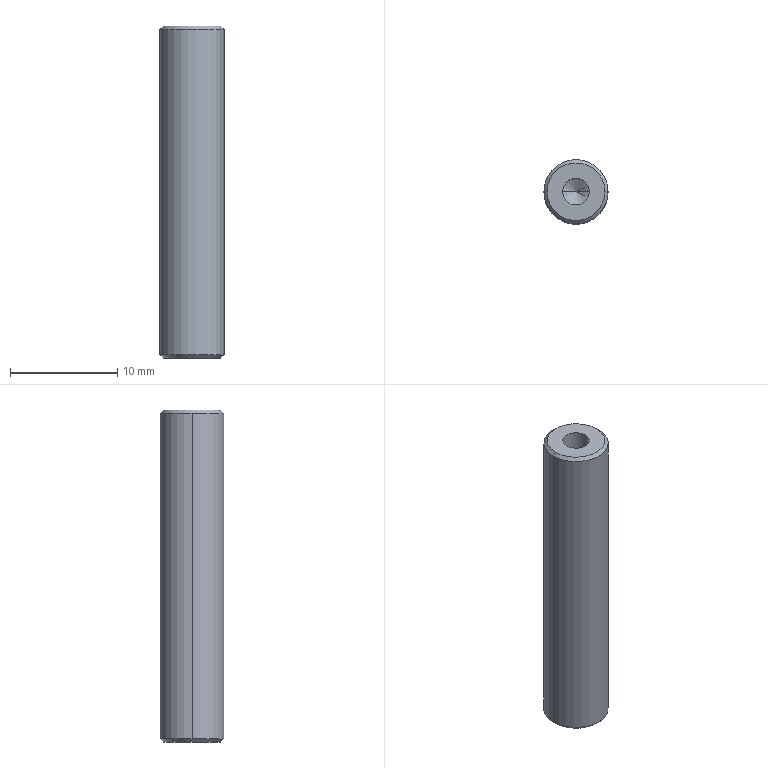Part | STEP file | 11-FG-SB01411 | 1 solid | 16 faces | box 6 x 6 x 31 mm | volume 798.775 mm3 | cone 8 | cylinder 6 | plane 2 | commonest cylinder face diameters 2.5 x4 6 x2
STEP:
#1=CARTESIAN_POINT('',(-2.7,0.,0.));
#2=VERTEX_POINT('',#1);
#3=CARTESIAN_POINT('',(2.7,0.,0.));
#4=VERTEX_POINT('',#3);
#5=CARTESIAN_POINT('',(0.,0.,0.));
#6=DIRECTION('',(0.,0.,-1.));
#7=DIRECTION('',(1.,0.,0.));
#8=AXIS2_PLACEMENT_3D('',#5,#6,#7);
#9=CIRCLE('',#8,2.7);
#10=EDGE_CURVE('',#2,#4,#9,.T.);
#11=ORIENTED_EDGE('',*,*,#10,.F.);
#12=CARTESIAN_POINT('',(-3.,0.,0.3));
#13=VERTEX_POINT('',#12);
#14=CARTESIAN_POINT('',(-3.,0.,0.3));
#15=DIRECTION('',(-0.7071,0.,0.7071));
#16=VECTOR('',#15,1000.);
#17=LINE('',#14,#16);
#18=EDGE_CURVE('',#2,#13,#17,.T.);
#19=ORIENTED_EDGE('',*,*,#18,.T.);
#20=CARTESIAN_POINT('',(3.,0.,0.3));
#21=VERTEX_POINT('',#20);
#22=CARTESIAN_POINT('',(0.,0.,0.3));
#23=DIRECTION('',(0.,0.,1.));
#24=DIRECTION('',(1.,0.,0.));
#25=AXIS2_PLACEMENT_3D('',#22,#23,#24);
#26=CIRCLE('',#25,3.);
#27=EDGE_CURVE('',#21,#13,#26,.T.);
#28=ORIENTED_EDGE('',*,*,#27,.F.);
#29=CARTESIAN_POINT('',(3.,0.,0.3));
#30=DIRECTION('',(0.7071,0.,0.7071));
#31=VECTOR('',#30,1000.);
#32=LINE('',#29,#31);
#33=EDGE_CURVE('',#4,#21,#32,.T.);
#34=ORIENTED_EDGE('',*,*,#33,.F.);
#35=EDGE_LOOP('',(#11,#19,#28,#34));
#36=FACE_OUTER_BOUND('',#35,.T.);
#37=CARTESIAN_POINT('',(0.,0.,0.3));
#38=DIRECTION('',(0.,0.,1.));
#39=DIRECTION('',(1.,0.,0.));
#40=AXIS2_PLACEMENT_3D('',#37,#38,#39);
#41=CONICAL_SURFACE('',#40,3.,0.7854);
#42=ADVANCED_FACE('',(#36),#41,.T.);
#43=CARTESIAN_POINT('',(2.7,0.,31.));
#44=VERTEX_POINT('',#43);
#45=CARTESIAN_POINT('',(-2.7,0.,31.));
#46=VERTEX_POINT('',#45);
#47=CARTESIAN_POINT('',(0.,0.,31.));
#48=DIRECTION('',(0.,0.,1.));
#49=DIRECTION('',(1.,0.,0.));
#50=AXIS2_PLACEMENT_3D('',#47,#48,#49);
#51=CIRCLE('',#50,2.7);
#52=EDGE_CURVE('',#44,#46,#51,.T.);
#53=ORIENTED_EDGE('',*,*,#52,.F.);
#54=CARTESIAN_POINT('',(3.,0.,30.7));
#55=VERTEX_POINT('',#54);
#56=CARTESIAN_POINT('',(2.7,0.,31.));
#57=DIRECTION('',(0.7071,0.,-0.7071));
#58=VECTOR('',#57,1000.);
#59=LINE('',#56,#58);
#60=EDGE_CURVE('',#44,#55,#59,.T.);
#61=ORIENTED_EDGE('',*,*,#60,.T.);
#62=CARTESIAN_POINT('',(-3.,0.,30.7));
#63=VERTEX_POINT('',#62);
#64=CARTESIAN_POINT('',(0.,0.,30.7));
#65=DIRECTION('',(0.,0.,-1.));
#66=DIRECTION('',(1.,0.,0.));
#67=AXIS2_PLACEMENT_3D('',#64,#65,#66);
#68=CIRCLE('',#67,3.);
#69=EDGE_CURVE('',#63,#55,#68,.T.);
#70=ORIENTED_EDGE('',*,*,#69,.F.);
#71=CARTESIAN_POINT('',(-2.7,0.,31.));
#72=DIRECTION('',(-0.7071,0.,-0.7071));
#73=VECTOR('',#72,1000.);
#74=LINE('',#71,#73);
#75=EDGE_CURVE('',#46,#63,#74,.T.);
#76=ORIENTED_EDGE('',*,*,#75,.F.);
#77=EDGE_LOOP('',(#53,#61,#70,#76));
#78=FACE_OUTER_BOUND('',#77,.T.);
#79=CARTESIAN_POINT('',(0.,0.,31.));
#80=DIRECTION('',(0.,0.,-1.));
#81=DIRECTION('',(-1.,0.,0.));
#82=AXIS2_PLACEMENT_3D('',#79,#80,#81);
#83=CONICAL_SURFACE('',#82,2.7,0.7854);
#84=ADVANCED_FACE('',(#78),#83,.T.);
#85=CARTESIAN_POINT('',(1.25,0.,7.5));
#86=VERTEX_POINT('',#85);
#87=CARTESIAN_POINT('',(-1.25,0.,7.5));
#88=VERTEX_POINT('',#87);
#89=CARTESIAN_POINT('',(0.,0.,7.5));
#90=DIRECTION('',(0.,0.,-1.));
#91=DIRECTION('',(-1.,0.,0.));
#92=AXIS2_PLACEMENT_3D('',#89,#90,#91);
#93=CIRCLE('',#92,1.25);
#94=EDGE_CURVE('',#86,#88,#93,.T.);
#95=ORIENTED_EDGE('',*,*,#94,.F.);
#96=CARTESIAN_POINT('',(1.25,0.,0.));
#97=VERTEX_POINT('',#96);
#98=CARTESIAN_POINT('',(1.25,0.,0.));
#99=DIRECTION('',(0.,0.,-1.));
#100=VECTOR('',#99,1000.);
#101=LINE('',#98,#100);
#102=EDGE_CURVE('',#86,#97,#101,.T.);
#103=ORIENTED_EDGE('',*,*,#102,.T.);
#104=CARTESIAN_POINT('',(-1.25,0.,0.));
#105=VERTEX_POINT('',#104);
#106=CARTESIAN_POINT('',(0.,0.,0.));
#107=DIRECTION('',(0.,0.,-1.));
#108=DIRECTION('',(-1.,0.,0.));
#109=AXIS2_PLACEMENT_3D('',#106,#107,#108);
#110=CIRCLE('',#109,1.25);
#111=EDGE_CURVE('',#97,#105,#110,.T.);
#112=ORIENTED_EDGE('',*,*,#111,.T.);
#113=CARTESIAN_POINT('',(-1.25,0.,0.));
#114=DIRECTION('',(0.,0.,-1.));
#115=VECTOR('',#114,1000.);
#116=LINE('',#113,#115);
#117=EDGE_CURVE('',#88,#105,#116,.T.);
#118=ORIENTED_EDGE('',*,*,#117,.F.);
#119=EDGE_LOOP('',(#95,#103,#112,#118));
#120=FACE_OUTER_BOUND('',#119,.T.);
#121=CARTESIAN_POINT('',(0.,0.,0.));
#122=DIRECTION('',(0.,0.,-1.));
#123=DIRECTION('',(-1.,0.,0.));
#124=AXIS2_PLACEMENT_3D('',#121,#122,#123);
#125=CYLINDRICAL_SURFACE('',#124,1.25);
#126=ADVANCED_FACE('',(#120),#125,.F.);
#127=CARTESIAN_POINT('',(0.,0.,8.251));
#128=VERTEX_POINT('',#127);
#129=CARTESIAN_POINT('',(-1.25,0.,7.5));
#130=DIRECTION('',(-0.8572,0.,-0.515));
#131=VECTOR('',#130,1000.);
#132=LINE('',#129,#131);
#133=EDGE_CURVE('',#128,#88,#132,.T.);
#134=ORIENTED_EDGE('',*,*,#133,.F.);
#135=CARTESIAN_POINT('',(1.25,0.,7.5));
#136=DIRECTION('',(0.8572,0.,-0.515));
#137=VECTOR('',#136,1000.);
#138=LINE('',#135,#137);
#139=EDGE_CURVE('',#128,#86,#138,.T.);
#140=ORIENTED_EDGE('',*,*,#139,.T.);
#141=ORIENTED_EDGE('',*,*,#94,.T.);
#142=EDGE_LOOP('',(#134,#140,#141));
#143=FACE_OUTER_BOUND('',#142,.T.);
#144=CARTESIAN_POINT('',(0.,0.,7.5));
#145=DIRECTION('',(0.,0.,-1.));
#146=DIRECTION('',(-1.,0.,0.));
#147=AXIS2_PLACEMENT_3D('',#144,#145,#146);
#148=CONICAL_SURFACE('',#147,1.25,1.03);
#149=ADVANCED_FACE('',(#143),#148,.F.);
#150=CARTESIAN_POINT('',(-1.25,0.,23.5));
#151=VERTEX_POINT('',#150);
#152=CARTESIAN_POINT('',(1.25,0.,23.5));
#153=VERTEX_POINT('',#152);
#154=CARTESIAN_POINT('',(0.,0.,23.5));
#155=DIRECTION('',(0.,0.,1.));
#156=DIRECTION('',(1.,0.,0.));
#157=AXIS2_PLACEMENT_3D('',#154,#155,#156);
#158=CIRCLE('',#157,1.25);
#159=EDGE_CURVE('',#151,#153,#158,.T.);
#160=ORIENTED_EDGE('',*,*,#159,.F.);
#161=CARTESIAN_POINT('',(-1.25,0.,31.));
#162=VERTEX_POINT('',#161);
#163=CARTESIAN_POINT('',(-1.25,0.,31.));
#164=DIRECTION('',(0.,0.,1.));
#165=VECTOR('',#164,1000.);
#166=LINE('',#163,#165);
#167=EDGE_CURVE('',#151,#162,#166,.T.);
#168=ORIENTED_EDGE('',*,*,#167,.T.);
#169=CARTESIAN_POINT('',(1.25,0.,31.));
#170=VERTEX_POINT('',#169);
#171=CARTESIAN_POINT('',(0.,0.,31.));
#172=DIRECTION('',(0.,0.,1.));
#173=DIRECTION('',(1.,0.,0.));
#174=AXIS2_PLACEMENT_3D('',#171,#172,#173);
#175=CIRCLE('',#174,1.25);
#176=EDGE_CURVE('',#162,#170,#175,.T.);
#177=ORIENTED_EDGE('',*,*,#176,.T.);
#178=CARTESIAN_POINT('',(1.25,0.,31.));
#179=DIRECTION('',(0.,0.,1.));
#180=VECTOR('',#179,1000.);
#181=LINE('',#178,#180);
#182=EDGE_CURVE('',#153,#170,#181,.T.);
#183=ORIENTED_EDGE('',*,*,#182,.F.);
#184=EDGE_LOOP('',(#160,#168,#177,#183));
#185=FACE_OUTER_BOUND('',#184,.T.);
#186=CARTESIAN_POINT('',(0.,0.,31.));
#187=DIRECTION('',(0.,0.,1.));
#188=DIRECTION('',(1.,0.,0.));
#189=AXIS2_PLACEMENT_3D('',#186,#187,#188);
#190=CYLINDRICAL_SURFACE('',#189,1.25);
#191=ADVANCED_FACE('',(#185),#190,.F.);
#192=CARTESIAN_POINT('',(0.,0.,22.749));
#193=VERTEX_POINT('',#192);
#194=CARTESIAN_POINT('',(1.25,0.,23.5));
#195=DIRECTION('',(0.8572,0.,0.515));
#196=VECTOR('',#195,1000.);
#197=LINE('',#194,#196);
#198=EDGE_CURVE('',#193,#153,#197,.T.);
#199=ORIENTED_EDGE('',*,*,#198,.F.);
#200=CARTESIAN_POINT('',(-1.25,0.,23.5));
#201=DIRECTION('',(-0.8572,0.,0.515));
#202=VECTOR('',#201,1000.);
#203=LINE('',#200,#202);
#204=EDGE_CURVE('',#193,#151,#203,.T.);
#205=ORIENTED_EDGE('',*,*,#204,.T.);
#206=ORIENTED_EDGE('',*,*,#159,.T.);
#207=EDGE_LOOP('',(#199,#205,#206));
#208=FACE_OUTER_BOUND('',#207,.T.);
#209=CARTESIAN_POINT('',(0.,0.,23.5));
#210=DIRECTION('',(0.,0.,1.));
#211=DIRECTION('',(1.,0.,0.));
#212=AXIS2_PLACEMENT_3D('',#209,#210,#211);
#213=CONICAL_SURFACE('',#212,1.25,1.03);
#214=ADVANCED_FACE('',(#208),#213,.F.);
#215=ORIENTED_EDGE('',*,*,#69,.T.);
#216=CARTESIAN_POINT('',(3.,0.,31.));
#217=DIRECTION('',(0.,0.,-1.));
#218=VECTOR('',#217,1000.);
#219=LINE('',#216,#218);
#220=EDGE_CURVE('',#55,#21,#219,.T.);
#221=ORIENTED_EDGE('',*,*,#220,.T.);
#222=ORIENTED_EDGE('',*,*,#27,.T.);
#223=CARTESIAN_POINT('',(-3.,0.,31.));
#224=DIRECTION('',(0.,0.,-1.));
#225=VECTOR('',#224,1000.);
#226=LINE('',#223,#225);
#227=EDGE_CURVE('',#63,#13,#226,.T.);
#228=ORIENTED_EDGE('',*,*,#227,.F.);
#229=EDGE_LOOP('',(#215,#221,#222,#228));
#230=FACE_OUTER_BOUND('',#229,.T.);
#231=CARTESIAN_POINT('',(0.,0.,31.));
#232=DIRECTION('',(0.,0.,-1.));
#233=DIRECTION('',(-1.,0.,0.));
#234=AXIS2_PLACEMENT_3D('',#231,#232,#233);
#235=CYLINDRICAL_SURFACE('',#234,3.);
#236=ADVANCED_FACE('',(#230),#235,.T.);
#237=ORIENTED_EDGE('',*,*,#220,.F.);
#238=CARTESIAN_POINT('',(0.,0.,30.7));
#239=DIRECTION('',(0.,0.,-1.));
#240=DIRECTION('',(1.,0.,0.));
#241=AXIS2_PLACEMENT_3D('',#238,#239,#240);
#242=CIRCLE('',#241,3.);
#243=EDGE_CURVE('',#55,#63,#242,.T.);
#244=ORIENTED_EDGE('',*,*,#243,.T.);
#245=ORIENTED_EDGE('',*,*,#227,.T.);
#246=CARTESIAN_POINT('',(0.,0.,0.3));
#247=DIRECTION('',(0.,0.,1.));
#248=DIRECTION('',(1.,0.,0.));
#249=AXIS2_PLACEMENT_3D('',#246,#247,#248);
#250=CIRCLE('',#249,3.);
#251=EDGE_CURVE('',#13,#21,#250,.T.);
#252=ORIENTED_EDGE('',*,*,#251,.T.);
#253=EDGE_LOOP('',(#237,#244,#245,#252));
#254=FACE_OUTER_BOUND('',#253,.T.);
#255=CARTESIAN_POINT('',(0.,0.,31.));
#256=DIRECTION('',(0.,0.,-1.));
#257=DIRECTION('',(-1.,0.,0.));
#258=AXIS2_PLACEMENT_3D('',#255,#256,#257);
#259=CYLINDRICAL_SURFACE('',#258,3.);
#260=ADVANCED_FACE('',(#254),#259,.T.);
#261=CARTESIAN_POINT('',(0.,0.,31.));
#262=DIRECTION('',(0.,0.,1.));
#263=DIRECTION('',(1.,0.,0.));
#264=AXIS2_PLACEMENT_3D('',#261,#262,#263);
#265=CIRCLE('',#264,2.7);
#266=EDGE_CURVE('',#46,#44,#265,.T.);
#267=ORIENTED_EDGE('',*,*,#266,.T.);
#268=ORIENTED_EDGE('',*,*,#52,.T.);
#269=EDGE_LOOP('',(#267,#268));
#270=FACE_OUTER_BOUND('',#269,.T.);
#271=CARTESIAN_POINT('',(0.,0.,31.));
#272=DIRECTION('',(0.,0.,1.));
#273=DIRECTION('',(1.,0.,0.));
#274=AXIS2_PLACEMENT_3D('',#271,#272,#273);
#275=CIRCLE('',#274,1.25);
#276=EDGE_CURVE('',#170,#162,#275,.T.);
#277=ORIENTED_EDGE('',*,*,#276,.F.);
#278=ORIENTED_EDGE('',*,*,#176,.F.);
#279=EDGE_LOOP('',(#277,#278));
#280=FACE_BOUND('',#279,.T.);
#281=CARTESIAN_POINT('',(0.,0.,31.));
#282=DIRECTION('',(0.,0.,1.));
#283=DIRECTION('',(1.,0.,0.));
#284=AXIS2_PLACEMENT_3D('',#281,#282,#283);
#285=PLANE('',#284);
#286=ADVANCED_FACE('',(#270,#280),#285,.T.);
#287=CARTESIAN_POINT('',(0.,0.,0.));
#288=DIRECTION('',(0.,0.,-1.));
#289=DIRECTION('',(1.,0.,0.));
#290=AXIS2_PLACEMENT_3D('',#287,#288,#289);
#291=CIRCLE('',#290,2.7);
#292=EDGE_CURVE('',#4,#2,#291,.T.);
#293=ORIENTED_EDGE('',*,*,#292,.T.);
#294=ORIENTED_EDGE('',*,*,#10,.T.);
#295=EDGE_LOOP('',(#293,#294));
#296=FACE_OUTER_BOUND('',#295,.T.);
#297=CARTESIAN_POINT('',(0.,0.,0.));
#298=DIRECTION('',(0.,0.,-1.));
#299=DIRECTION('',(-1.,0.,0.));
#300=AXIS2_PLACEMENT_3D('',#297,#298,#299);
#301=CIRCLE('',#300,1.25);
#302=EDGE_CURVE('',#105,#97,#301,.T.);
#303=ORIENTED_EDGE('',*,*,#302,.F.);
#304=ORIENTED_EDGE('',*,*,#111,.F.);
#305=EDGE_LOOP('',(#303,#304));
#306=FACE_BOUND('',#305,.T.);
#307=CARTESIAN_POINT('',(0.,0.,0.));
#308=DIRECTION('',(0.,0.,1.));
#309=DIRECTION('',(1.,0.,0.));
#310=AXIS2_PLACEMENT_3D('',#307,#308,#309);
#311=PLANE('',#310);
#312=ADVANCED_FACE('',(#296,#306),#311,.F.);
#313=ORIENTED_EDGE('',*,*,#204,.F.);
#314=ORIENTED_EDGE('',*,*,#198,.T.);
#315=CARTESIAN_POINT('',(0.,0.,23.5));
#316=DIRECTION('',(0.,0.,1.));
#317=DIRECTION('',(1.,0.,0.));
#318=AXIS2_PLACEMENT_3D('',#315,#316,#317);
#319=CIRCLE('',#318,1.25);
#320=EDGE_CURVE('',#153,#151,#319,.T.);
#321=ORIENTED_EDGE('',*,*,#320,.T.);
#322=EDGE_LOOP('',(#313,#314,#321));
#323=FACE_OUTER_BOUND('',#322,.T.);
#324=CARTESIAN_POINT('',(0.,0.,23.5));
#325=DIRECTION('',(0.,0.,1.));
#326=DIRECTION('',(1.,0.,0.));
#327=AXIS2_PLACEMENT_3D('',#324,#325,#326);
#328=CONICAL_SURFACE('',#327,1.25,1.03);
#329=ADVANCED_FACE('',(#323),#328,.F.);
#330=ORIENTED_EDGE('',*,*,#167,.F.);
#331=ORIENTED_EDGE('',*,*,#320,.F.);
#332=ORIENTED_EDGE('',*,*,#182,.T.);
#333=ORIENTED_EDGE('',*,*,#276,.T.);
#334=EDGE_LOOP('',(#330,#331,#332,#333));
#335=FACE_OUTER_BOUND('',#334,.T.);
#336=CARTESIAN_POINT('',(0.,0.,31.));
#337=DIRECTION('',(0.,0.,1.));
#338=DIRECTION('',(1.,0.,0.));
#339=AXIS2_PLACEMENT_3D('',#336,#337,#338);
#340=CYLINDRICAL_SURFACE('',#339,1.25);
#341=ADVANCED_FACE('',(#335),#340,.F.);
#342=ORIENTED_EDGE('',*,*,#139,.F.);
#343=ORIENTED_EDGE('',*,*,#133,.T.);
#344=CARTESIAN_POINT('',(0.,0.,7.5));
#345=DIRECTION('',(0.,0.,-1.));
#346=DIRECTION('',(-1.,0.,0.));
#347=AXIS2_PLACEMENT_3D('',#344,#345,#346);
#348=CIRCLE('',#347,1.25);
#349=EDGE_CURVE('',#88,#86,#348,.T.);
#350=ORIENTED_EDGE('',*,*,#349,.T.);
#351=EDGE_LOOP('',(#342,#343,#350));
#352=FACE_OUTER_BOUND('',#351,.T.);
#353=CARTESIAN_POINT('',(0.,0.,7.5));
#354=DIRECTION('',(0.,0.,-1.));
#355=DIRECTION('',(-1.,0.,0.));
#356=AXIS2_PLACEMENT_3D('',#353,#354,#355);
#357=CONICAL_SURFACE('',#356,1.25,1.03);
#358=ADVANCED_FACE('',(#352),#357,.F.);
#359=ORIENTED_EDGE('',*,*,#102,.F.);
#360=ORIENTED_EDGE('',*,*,#349,.F.);
#361=ORIENTED_EDGE('',*,*,#117,.T.);
#362=ORIENTED_EDGE('',*,*,#302,.T.);
#363=EDGE_LOOP('',(#359,#360,#361,#362));
#364=FACE_OUTER_BOUND('',#363,.T.);
#365=CARTESIAN_POINT('',(0.,0.,0.));
#366=DIRECTION('',(0.,0.,-1.));
#367=DIRECTION('',(-1.,0.,0.));
#368=AXIS2_PLACEMENT_3D('',#365,#366,#367);
#369=CYLINDRICAL_SURFACE('',#368,1.25);
#370=ADVANCED_FACE('',(#364),#369,.F.);
#371=ORIENTED_EDGE('',*,*,#60,.F.);
#372=ORIENTED_EDGE('',*,*,#266,.F.);
#373=ORIENTED_EDGE('',*,*,#75,.T.);
#374=ORIENTED_EDGE('',*,*,#243,.F.);
#375=EDGE_LOOP('',(#371,#372,#373,#374));
#376=FACE_OUTER_BOUND('',#375,.T.);
#377=CARTESIAN_POINT('',(0.,0.,31.));
#378=DIRECTION('',(0.,0.,-1.));
#379=DIRECTION('',(-1.,0.,0.));
#380=AXIS2_PLACEMENT_3D('',#377,#378,#379);
#381=CONICAL_SURFACE('',#380,2.7,0.7854);
#382=ADVANCED_FACE('',(#376),#381,.T.);
#383=ORIENTED_EDGE('',*,*,#18,.F.);
#384=ORIENTED_EDGE('',*,*,#292,.F.);
#385=ORIENTED_EDGE('',*,*,#33,.T.);
#386=ORIENTED_EDGE('',*,*,#251,.F.);
#387=EDGE_LOOP('',(#383,#384,#385,#386));
#388=FACE_OUTER_BOUND('',#387,.T.);
#389=CARTESIAN_POINT('',(0.,0.,0.3));
#390=DIRECTION('',(0.,0.,1.));
#391=DIRECTION('',(1.,0.,0.));
#392=AXIS2_PLACEMENT_3D('',#389,#390,#391);
#393=CONICAL_SURFACE('',#392,3.,0.7854);
#394=ADVANCED_FACE('',(#388),#393,.T.);
#395=CLOSED_SHELL('',(#42,#84,#126,#149,#191,#214,#236,#260,#286,#312,#329,#341,#358,#370,#382,#394));
#396=MANIFOLD_SOLID_BREP('',#395);
#397=CARTESIAN_POINT('',(0.,0.,0.));
#398=DIRECTION('',(0.,0.,1.));
#399=DIRECTION('',(1.,0.,0.));
#400=AXIS2_PLACEMENT_3D('',#397,#398,#399);
#401=(LENGTH_UNIT()NAMED_UNIT(*)SI_UNIT(.MILLI.,.METRE.));
#402=UNCERTAINTY_MEASURE_WITH_UNIT(LENGTH_MEASURE(0.00001),#401,'','');
#403=(NAMED_UNIT(*)PLANE_ANGLE_UNIT()SI_UNIT($,.RADIAN.));
#404=(NAMED_UNIT(*)SI_UNIT($,.STERADIAN.)SOLID_ANGLE_UNIT());
#405=(GEOMETRIC_REPRESENTATION_CONTEXT(3)GLOBAL_UNCERTAINTY_ASSIGNED_CONTEXT((#402))GLOBAL_UNIT_ASSIGNED_CONTEXT((#401,#403,#404))REPRESENTATION_CONTEXT('',''));
#406=ADVANCED_BREP_SHAPE_REPRESENTATION('',(#396,#400),#405);